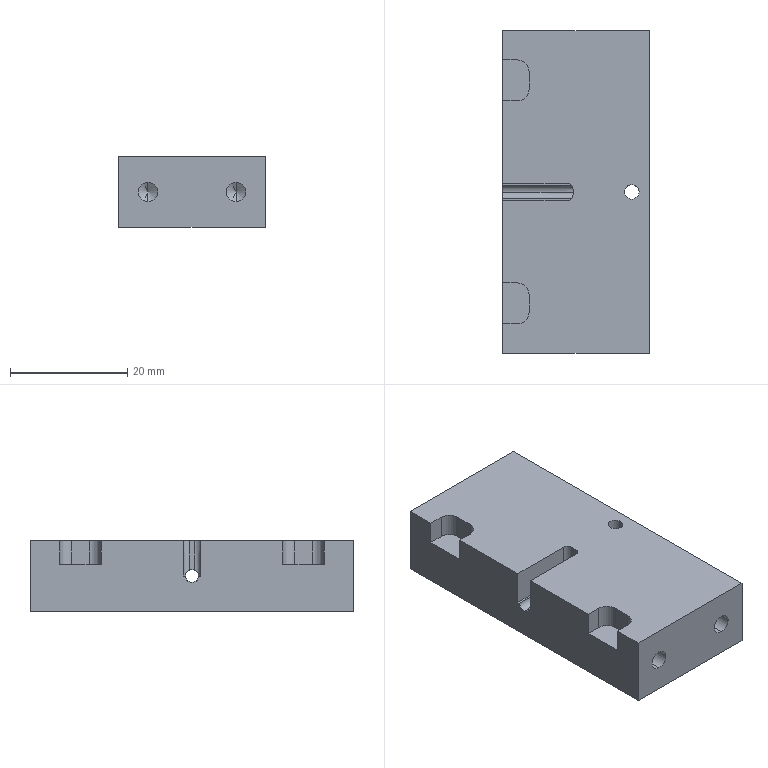Part | SolidWorks | features ICE 4, Chamfer 2, Fillet 2, HoleWzd 2, MirrorPattern 2, Extrusion 1 | 1 solid | 52 faces | box 25 x 55 x 12 mm | volume 15456 mm3 | cylinder 22 | plane 20 | cone 8 | torus 2 | commonest cylinder face diameters 3.3 x8 2.5 x4 4 x4 2 x2 2.2 x2 5 x2